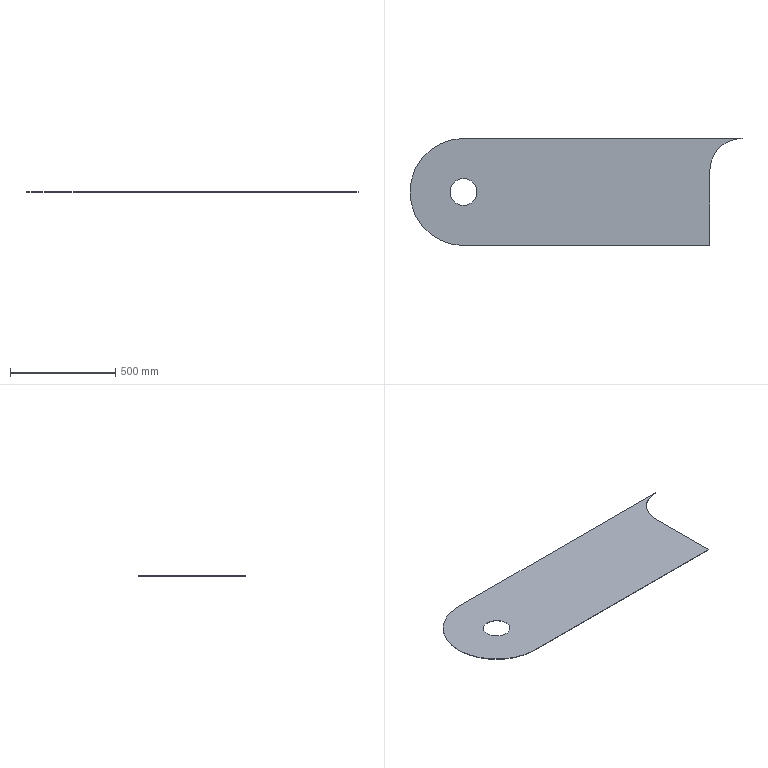Part | SolidWorks | features Extrusion 1 | 1 solid | 10 faces | box 1575 x 508 x 2 mm | volume 1374411 mm3 | cylinder 5 | plane 5 | commonest cylinder face diameters 127 x2 508 x2 304.8 x1
STEP:
#1=CARTESIAN_POINT('',(-63.5,0.,1.));
#2=VERTEX_POINT('',#1);
#3=CARTESIAN_POINT('',(63.5,0.,1.));
#4=VERTEX_POINT('',#3);
#5=CARTESIAN_POINT('',(0.,0.,1.));
#6=DIRECTION('',(0.,0.,1.));
#7=DIRECTION('',(1.,0.,0.));
#8=AXIS2_PLACEMENT_3D('',#5,#6,#7);
#9=CIRCLE('',#8,63.5);
#10=EDGE_CURVE('',#2,#4,#9,.T.);
#11=ORIENTED_EDGE('',*,*,#10,.T.);
#12=CARTESIAN_POINT('',(63.5,0.,-1.));
#13=VERTEX_POINT('',#12);
#14=CARTESIAN_POINT('',(63.5,0.,1.));
#15=DIRECTION('',(0.,0.,-1.));
#16=VECTOR('',#15,1000.);
#17=LINE('',#14,#16);
#18=EDGE_CURVE('',#4,#13,#17,.T.);
#19=ORIENTED_EDGE('',*,*,#18,.T.);
#20=CARTESIAN_POINT('',(-63.5,0.,-1.));
#21=VERTEX_POINT('',#20);
#22=CARTESIAN_POINT('',(0.,0.,-1.));
#23=DIRECTION('',(0.,0.,1.));
#24=DIRECTION('',(1.,0.,0.));
#25=AXIS2_PLACEMENT_3D('',#22,#23,#24);
#26=CIRCLE('',#25,63.5);
#27=EDGE_CURVE('',#21,#13,#26,.T.);
#28=ORIENTED_EDGE('',*,*,#27,.F.);
#29=CARTESIAN_POINT('',(-63.5,0.,1.));
#30=DIRECTION('',(0.,0.,-1.));
#31=VECTOR('',#30,1000.);
#32=LINE('',#29,#31);
#33=EDGE_CURVE('',#2,#21,#32,.T.);
#34=ORIENTED_EDGE('',*,*,#33,.F.);
#35=EDGE_LOOP('',(#11,#19,#28,#34));
#36=FACE_OUTER_BOUND('',#35,.T.);
#37=CARTESIAN_POINT('',(0.,0.,1.));
#38=DIRECTION('',(0.,0.,-1.));
#39=DIRECTION('',(-1.,0.,0.));
#40=AXIS2_PLACEMENT_3D('',#37,#38,#39);
#41=CYLINDRICAL_SURFACE('',#40,63.5);
#42=ADVANCED_FACE('',(#36),#41,.F.);
#43=CARTESIAN_POINT('',(-254.,0.,1.));
#44=VERTEX_POINT('',#43);
#45=CARTESIAN_POINT('',(0.,-254.,1.));
#46=VERTEX_POINT('',#45);
#47=CARTESIAN_POINT('',(0.,0.,1.));
#48=DIRECTION('',(0.,0.,1.));
#49=DIRECTION('',(1.,0.,0.));
#50=AXIS2_PLACEMENT_3D('',#47,#48,#49);
#51=CIRCLE('',#50,254.);
#52=EDGE_CURVE('',#44,#46,#51,.T.);
#53=ORIENTED_EDGE('',*,*,#52,.F.);
#54=CARTESIAN_POINT('',(-254.,0.,-1.));
#55=VERTEX_POINT('',#54);
#56=CARTESIAN_POINT('',(-254.,0.,1.));
#57=DIRECTION('',(0.,0.,-1.));
#58=VECTOR('',#57,1000.);
#59=LINE('',#56,#58);
#60=EDGE_CURVE('',#44,#55,#59,.T.);
#61=ORIENTED_EDGE('',*,*,#60,.T.);
#62=CARTESIAN_POINT('',(0.,-254.,-1.));
#63=VERTEX_POINT('',#62);
#64=CARTESIAN_POINT('',(0.,0.,-1.));
#65=DIRECTION('',(0.,0.,1.));
#66=DIRECTION('',(1.,0.,0.));
#67=AXIS2_PLACEMENT_3D('',#64,#65,#66);
#68=CIRCLE('',#67,254.);
#69=EDGE_CURVE('',#55,#63,#68,.T.);
#70=ORIENTED_EDGE('',*,*,#69,.T.);
#71=CARTESIAN_POINT('',(0.,-254.,1.));
#72=DIRECTION('',(0.,0.,-1.));
#73=VECTOR('',#72,1000.);
#74=LINE('',#71,#73);
#75=EDGE_CURVE('',#46,#63,#74,.T.);
#76=ORIENTED_EDGE('',*,*,#75,.F.);
#77=EDGE_LOOP('',(#53,#61,#70,#76));
#78=FACE_OUTER_BOUND('',#77,.T.);
#79=CARTESIAN_POINT('',(0.,0.,1.));
#80=DIRECTION('',(0.,0.,-1.));
#81=DIRECTION('',(-1.,0.,0.));
#82=AXIS2_PLACEMENT_3D('',#79,#80,#81);
#83=CYLINDRICAL_SURFACE('',#82,254.);
#84=ADVANCED_FACE('',(#78),#83,.T.);
#85=CARTESIAN_POINT('',(0.,254.,1.));
#86=VERTEX_POINT('',#85);
#87=CARTESIAN_POINT('',(0.,0.,1.));
#88=DIRECTION('',(0.,0.,1.));
#89=DIRECTION('',(1.,0.,0.));
#90=AXIS2_PLACEMENT_3D('',#87,#88,#89);
#91=CIRCLE('',#90,254.);
#92=EDGE_CURVE('',#86,#44,#91,.T.);
#93=ORIENTED_EDGE('',*,*,#92,.T.);
#94=ORIENTED_EDGE('',*,*,#52,.T.);
#95=CARTESIAN_POINT('',(1168.4,-254.,1.));
#96=VERTEX_POINT('',#95);
#97=CARTESIAN_POINT('',(0.,-254.,1.));
#98=DIRECTION('',(1.,0.,0.));
#99=VECTOR('',#98,1000.);
#100=LINE('',#97,#99);
#101=EDGE_CURVE('',#46,#96,#100,.T.);
#102=ORIENTED_EDGE('',*,*,#101,.T.);
#103=CARTESIAN_POINT('',(1168.4,101.6,1.));
#104=VERTEX_POINT('',#103);
#105=CARTESIAN_POINT('',(1168.4,-254.,1.));
#106=DIRECTION('',(0.,1.,0.));
#107=VECTOR('',#106,1000.);
#108=LINE('',#105,#107);
#109=EDGE_CURVE('',#96,#104,#108,.T.);
#110=ORIENTED_EDGE('',*,*,#109,.T.);
#111=CARTESIAN_POINT('',(1320.8,254.,1.));
#112=VERTEX_POINT('',#111);
#113=CARTESIAN_POINT('',(1320.8,101.6,1.));
#114=DIRECTION('',(0.,0.,-1.));
#115=DIRECTION('',(1.,0.,0.));
#116=AXIS2_PLACEMENT_3D('',#113,#114,#115);
#117=CIRCLE('',#116,152.4);
#118=EDGE_CURVE('',#104,#112,#117,.T.);
#119=ORIENTED_EDGE('',*,*,#118,.T.);
#120=CARTESIAN_POINT('',(0.,254.,1.));
#121=DIRECTION('',(-1.,0.,0.));
#122=VECTOR('',#121,1000.);
#123=LINE('',#120,#122);
#124=EDGE_CURVE('',#112,#86,#123,.T.);
#125=ORIENTED_EDGE('',*,*,#124,.T.);
#126=EDGE_LOOP('',(#93,#94,#102,#110,#119,#125));
#127=FACE_OUTER_BOUND('',#126,.T.);
#128=ORIENTED_EDGE('',*,*,#10,.F.);
#129=CARTESIAN_POINT('',(0.,0.,1.));
#130=DIRECTION('',(0.,0.,1.));
#131=DIRECTION('',(1.,0.,0.));
#132=AXIS2_PLACEMENT_3D('',#129,#130,#131);
#133=CIRCLE('',#132,63.5);
#134=EDGE_CURVE('',#4,#2,#133,.T.);
#135=ORIENTED_EDGE('',*,*,#134,.F.);
#136=EDGE_LOOP('',(#128,#135));
#137=FACE_BOUND('',#136,.T.);
#138=CARTESIAN_POINT('',(0.,0.,1.));
#139=DIRECTION('',(0.,0.,1.));
#140=DIRECTION('',(1.,0.,0.));
#141=AXIS2_PLACEMENT_3D('',#138,#139,#140);
#142=PLANE('',#141);
#143=ADVANCED_FACE('',(#127,#137),#142,.T.);
#144=CARTESIAN_POINT('',(0.,254.,-1.));
#145=VERTEX_POINT('',#144);
#146=CARTESIAN_POINT('',(0.,0.,-1.));
#147=DIRECTION('',(0.,0.,1.));
#148=DIRECTION('',(1.,0.,0.));
#149=AXIS2_PLACEMENT_3D('',#146,#147,#148);
#150=CIRCLE('',#149,254.);
#151=EDGE_CURVE('',#145,#55,#150,.T.);
#152=ORIENTED_EDGE('',*,*,#151,.F.);
#153=CARTESIAN_POINT('',(1320.8,254.,-1.));
#154=VERTEX_POINT('',#153);
#155=CARTESIAN_POINT('',(0.,254.,-1.));
#156=DIRECTION('',(-1.,0.,0.));
#157=VECTOR('',#156,1000.);
#158=LINE('',#155,#157);
#159=EDGE_CURVE('',#154,#145,#158,.T.);
#160=ORIENTED_EDGE('',*,*,#159,.F.);
#161=CARTESIAN_POINT('',(1168.4,101.6,-1.));
#162=VERTEX_POINT('',#161);
#163=CARTESIAN_POINT('',(1320.8,101.6,-1.));
#164=DIRECTION('',(0.,0.,-1.));
#165=DIRECTION('',(1.,0.,0.));
#166=AXIS2_PLACEMENT_3D('',#163,#164,#165);
#167=CIRCLE('',#166,152.4);
#168=EDGE_CURVE('',#162,#154,#167,.T.);
#169=ORIENTED_EDGE('',*,*,#168,.F.);
#170=CARTESIAN_POINT('',(1168.4,-254.,-1.));
#171=VERTEX_POINT('',#170);
#172=CARTESIAN_POINT('',(1168.4,-254.,-1.));
#173=DIRECTION('',(0.,1.,0.));
#174=VECTOR('',#173,1000.);
#175=LINE('',#172,#174);
#176=EDGE_CURVE('',#171,#162,#175,.T.);
#177=ORIENTED_EDGE('',*,*,#176,.F.);
#178=CARTESIAN_POINT('',(0.,-254.,-1.));
#179=DIRECTION('',(1.,0.,0.));
#180=VECTOR('',#179,1000.);
#181=LINE('',#178,#180);
#182=EDGE_CURVE('',#63,#171,#181,.T.);
#183=ORIENTED_EDGE('',*,*,#182,.F.);
#184=ORIENTED_EDGE('',*,*,#69,.F.);
#185=EDGE_LOOP('',(#152,#160,#169,#177,#183,#184));
#186=FACE_OUTER_BOUND('',#185,.T.);
#187=ORIENTED_EDGE('',*,*,#27,.T.);
#188=CARTESIAN_POINT('',(0.,0.,-1.));
#189=DIRECTION('',(0.,0.,1.));
#190=DIRECTION('',(1.,0.,0.));
#191=AXIS2_PLACEMENT_3D('',#188,#189,#190);
#192=CIRCLE('',#191,63.5);
#193=EDGE_CURVE('',#13,#21,#192,.T.);
#194=ORIENTED_EDGE('',*,*,#193,.T.);
#195=EDGE_LOOP('',(#187,#194));
#196=FACE_BOUND('',#195,.T.);
#197=CARTESIAN_POINT('',(0.,0.,-1.));
#198=DIRECTION('',(0.,0.,1.));
#199=DIRECTION('',(1.,0.,0.));
#200=AXIS2_PLACEMENT_3D('',#197,#198,#199);
#201=PLANE('',#200);
#202=ADVANCED_FACE('',(#186,#196),#201,.F.);
#203=ORIENTED_EDGE('',*,*,#60,.F.);
#204=ORIENTED_EDGE('',*,*,#92,.F.);
#205=CARTESIAN_POINT('',(0.,254.,1.));
#206=DIRECTION('',(0.,0.,-1.));
#207=VECTOR('',#206,1000.);
#208=LINE('',#205,#207);
#209=EDGE_CURVE('',#86,#145,#208,.T.);
#210=ORIENTED_EDGE('',*,*,#209,.T.);
#211=ORIENTED_EDGE('',*,*,#151,.T.);
#212=EDGE_LOOP('',(#203,#204,#210,#211));
#213=FACE_OUTER_BOUND('',#212,.T.);
#214=CARTESIAN_POINT('',(0.,0.,1.));
#215=DIRECTION('',(0.,0.,-1.));
#216=DIRECTION('',(-1.,0.,0.));
#217=AXIS2_PLACEMENT_3D('',#214,#215,#216);
#218=CYLINDRICAL_SURFACE('',#217,254.);
#219=ADVANCED_FACE('',(#213),#218,.T.);
#220=ORIENTED_EDGE('',*,*,#182,.T.);
#221=CARTESIAN_POINT('',(1168.4,-254.,1.));
#222=DIRECTION('',(0.,0.,-1.));
#223=VECTOR('',#222,1000.);
#224=LINE('',#221,#223);
#225=EDGE_CURVE('',#96,#171,#224,.T.);
#226=ORIENTED_EDGE('',*,*,#225,.F.);
#227=ORIENTED_EDGE('',*,*,#101,.F.);
#228=ORIENTED_EDGE('',*,*,#75,.T.);
#229=EDGE_LOOP('',(#220,#226,#227,#228));
#230=FACE_OUTER_BOUND('',#229,.T.);
#231=CARTESIAN_POINT('',(0.,-254.,1.));
#232=DIRECTION('',(0.,1.,0.));
#233=DIRECTION('',(0.,0.,1.));
#234=AXIS2_PLACEMENT_3D('',#231,#232,#233);
#235=PLANE('',#234);
#236=ADVANCED_FACE('',(#230),#235,.F.);
#237=ORIENTED_EDGE('',*,*,#176,.T.);
#238=CARTESIAN_POINT('',(1168.4,101.6,1.));
#239=DIRECTION('',(0.,0.,-1.));
#240=VECTOR('',#239,1000.);
#241=LINE('',#238,#240);
#242=EDGE_CURVE('',#104,#162,#241,.T.);
#243=ORIENTED_EDGE('',*,*,#242,.F.);
#244=ORIENTED_EDGE('',*,*,#109,.F.);
#245=ORIENTED_EDGE('',*,*,#225,.T.);
#246=EDGE_LOOP('',(#237,#243,#244,#245));
#247=FACE_OUTER_BOUND('',#246,.T.);
#248=CARTESIAN_POINT('',(1168.4,-254.,1.));
#249=DIRECTION('',(-1.,0.,0.));
#250=DIRECTION('',(0.,0.,1.));
#251=AXIS2_PLACEMENT_3D('',#248,#249,#250);
#252=PLANE('',#251);
#253=ADVANCED_FACE('',(#247),#252,.F.);
#254=ORIENTED_EDGE('',*,*,#168,.T.);
#255=CARTESIAN_POINT('',(1320.8,254.,1.));
#256=DIRECTION('',(0.,0.,-1.));
#257=VECTOR('',#256,1000.);
#258=LINE('',#255,#257);
#259=EDGE_CURVE('',#112,#154,#258,.T.);
#260=ORIENTED_EDGE('',*,*,#259,.F.);
#261=ORIENTED_EDGE('',*,*,#118,.F.);
#262=ORIENTED_EDGE('',*,*,#242,.T.);
#263=EDGE_LOOP('',(#254,#260,#261,#262));
#264=FACE_OUTER_BOUND('',#263,.T.);
#265=CARTESIAN_POINT('',(1320.8,101.6,1.));
#266=DIRECTION('',(0.,0.,-1.));
#267=DIRECTION('',(-1.,0.,0.));
#268=AXIS2_PLACEMENT_3D('',#265,#266,#267);
#269=CYLINDRICAL_SURFACE('',#268,152.4);
#270=ADVANCED_FACE('',(#264),#269,.F.);
#271=ORIENTED_EDGE('',*,*,#159,.T.);
#272=ORIENTED_EDGE('',*,*,#209,.F.);
#273=ORIENTED_EDGE('',*,*,#124,.F.);
#274=ORIENTED_EDGE('',*,*,#259,.T.);
#275=EDGE_LOOP('',(#271,#272,#273,#274));
#276=FACE_OUTER_BOUND('',#275,.T.);
#277=CARTESIAN_POINT('',(0.,254.,1.));
#278=DIRECTION('',(0.,-1.,0.));
#279=DIRECTION('',(0.,0.,-1.));
#280=AXIS2_PLACEMENT_3D('',#277,#278,#279);
#281=PLANE('',#280);
#282=ADVANCED_FACE('',(#276),#281,.F.);
#283=ORIENTED_EDGE('',*,*,#18,.F.);
#284=ORIENTED_EDGE('',*,*,#134,.T.);
#285=ORIENTED_EDGE('',*,*,#33,.T.);
#286=ORIENTED_EDGE('',*,*,#193,.F.);
#287=EDGE_LOOP('',(#283,#284,#285,#286));
#288=FACE_OUTER_BOUND('',#287,.T.);
#289=CARTESIAN_POINT('',(0.,0.,1.));
#290=DIRECTION('',(0.,0.,-1.));
#291=DIRECTION('',(-1.,0.,0.));
#292=AXIS2_PLACEMENT_3D('',#289,#290,#291);
#293=CYLINDRICAL_SURFACE('',#292,63.5);
#294=ADVANCED_FACE('',(#288),#293,.F.);
#295=CLOSED_SHELL('',(#42,#84,#143,#202,#219,#236,#253,#270,#282,#294));
#296=MANIFOLD_SOLID_BREP('',#295);
#297=CARTESIAN_POINT('',(0.,0.,0.));
#298=DIRECTION('',(0.,0.,1.));
#299=DIRECTION('',(1.,0.,0.));
#300=AXIS2_PLACEMENT_3D('',#297,#298,#299);
#301=(LENGTH_UNIT()NAMED_UNIT(*)SI_UNIT(.MILLI.,.METRE.));
#302=UNCERTAINTY_MEASURE_WITH_UNIT(LENGTH_MEASURE(0.00001),#301,'','');
#303=(NAMED_UNIT(*)PLANE_ANGLE_UNIT()SI_UNIT($,.RADIAN.));
#304=(NAMED_UNIT(*)SI_UNIT($,.STERADIAN.)SOLID_ANGLE_UNIT());
#305=(GEOMETRIC_REPRESENTATION_CONTEXT(3)GLOBAL_UNCERTAINTY_ASSIGNED_CONTEXT((#302))GLOBAL_UNIT_ASSIGNED_CONTEXT((#301,#303,#304))REPRESENTATION_CONTEXT('',''));
#306=ADVANCED_BREP_SHAPE_REPRESENTATION('',(#296,#300),#305);